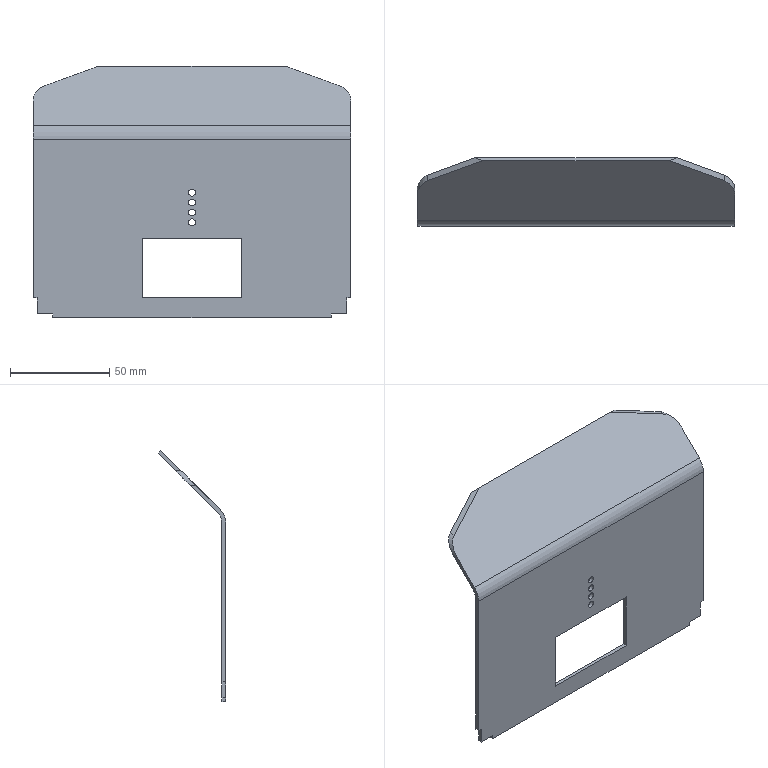Part | STEP file | 1-43.6 | 1 solid | 30 faces | box 160 x 34.183 x 126.611 mm | volume 40223 mm3 | plane 22 | cylinder 8 | commonest cylinder face diameters 3.5 x4 16 x3 20 x1